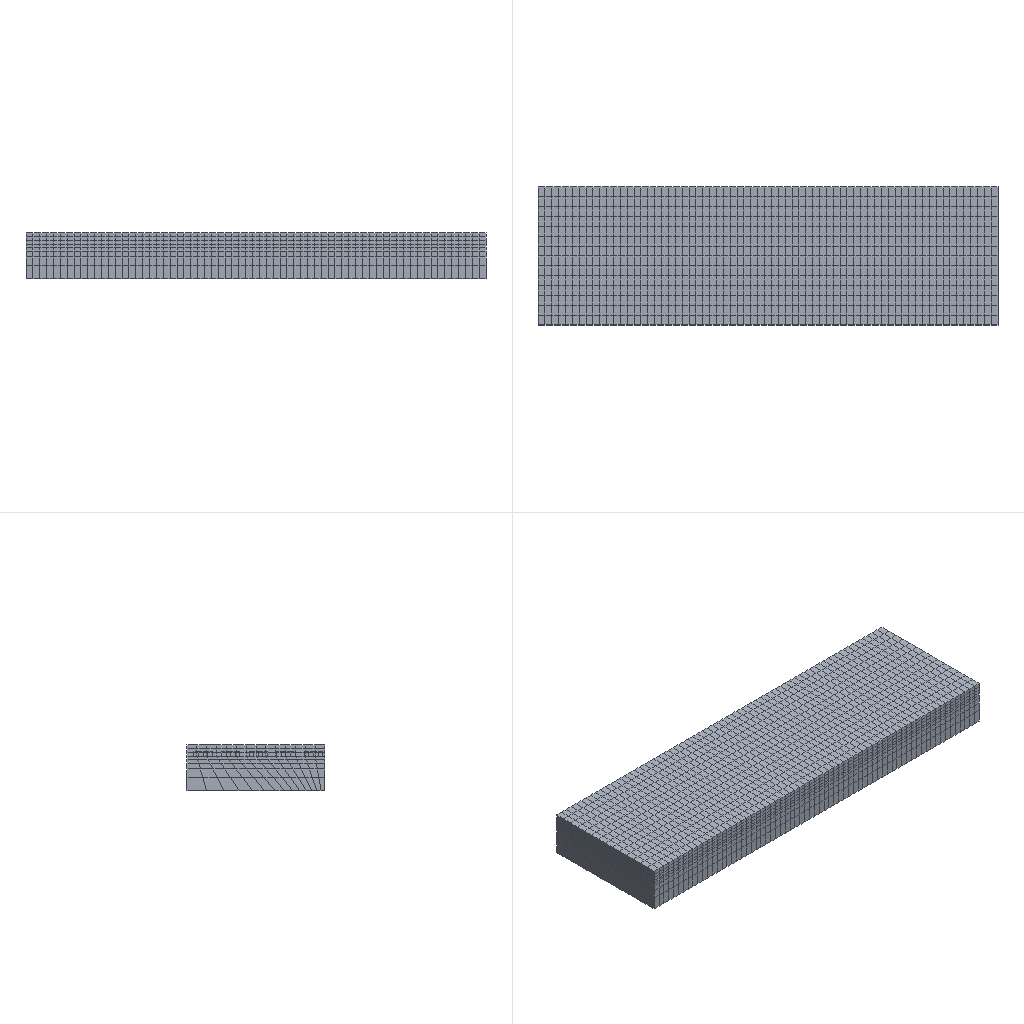Simulation study | abaqus
Set-up summary:
category,name,step,type,value,unit,region
solver,abaqus
solver,version,,,Abaqus/Explicit 2020
units,not stated in the deck,,not stated
analysis,deck,,transient,transient
load_step,Step-1,Step-1,transient
load_step,requested,,,1
mesh,nodes,,,14180
mesh,elements,,,9725
element_type,R3D3,,rigid,228
element_type,R3D4,,rigid,633
element_type,C3D8R,,solid,1360
element_type,EC3D8R,,solid,7504
load,load commands in deck,,count,1
bc,support commands in deck,,count,10
material,BING,,in results
material,COH,,in results
material,WATER,,in results
check,setup vs results,,match,"per instance, exact: element labels, types and connectivity; labels of the nodes the elements use; coordinates of those nodes at SINGLE_PRECISION in 86 of 87 instance(s)"
Abaqus input file, long lists of numbers shortened:
*Heading
** Job name: Job-3 Model name: Model-1-Copy-Copy
** Generated by: Abaqus/CAE 2020
*Preprint, echo=NO, model=NO, history=NO, contact=NO
**
** PARTS
**
*Part, name=aa
*Node
      1,           0.,        -400.,         100.
      2,           0.,        -300.,         100.
** (48 more lines like these left out)
*Element, type=C3D8R
 1, 11, 12, 17, 16,  1,  2,  7,  6
 2, 12, 13, 18, 17,  2,  3,  8,  7
** (14 more lines like these left out)
*Nset, nset=Set-1, generate
  1,  50,   1
*Elset, elset=Set-1, generate
  1,  16,   1
** Section: bing
*Solid Section, elset=Set-1, material=bing
,
*End Part
**
*Part, name=oula
*Node
      1,       10000.,           0.,         750.
      2,       10000.,       -3000.,         750.
** (9178 more lines like these left out)
*Element, type=EC3D8R
   1,  212, 1143, 4033,  615,    1,   13,  511,   46
   2, 1143, 1144, 4034, 4033,   13,   14,  512,  511
** (7502 more lines like these left out)
*Nset, nset=Set-1, generate
    1,  9180,     1
*Elset, elset=Set-1, generate
    1,  7504,     1
** Section: oula
*Eulerian Section, elset=Set-1
water, water-1
*Surface, type=EULERIAN MATERIAL, name=water-1
water-1
*End Part
**
*Part, name=work
*Node
      1,    2.375,   6757.633,   37190.746
      2,    2.375,   6757.633,   40618.258
** (747 more lines like these left out)
*Element, type=R3D4
 1,  1, 21, 64,  4
 2, 21, 22, 63, 64
** (631 more lines like these left out)
*Element, type=R3D3
369,  4, 65,  5
370, 71, 59, 58
** (226 more lines like these left out)
*Node
    750,    2.375,   6959.508,   38910.039
*Nset, nset=work-RefPt_, internal
750,
*Elset, elset=work, generate
   1,  861,    1
*End Part
**
**
** ASSEMBLY
**
*Assembly, name=Assembly
**
*Instance, name=work-1, part=work
37076.822, -1497.625, -5616.383
37076.822, -1497.625, -5616.383, 37077.399, -1498.203, -5616.96,         120.
*End Instance
**
*Instance, name=oula-1, part=oula
          0.,           0.,         250.
*End Instance
**
*Instance, name=aa-1, part=aa
       9600.,       -2550.,        1000.
*End Instance
**
*Instance, name=aa-1-lin-1-2, part=aa
       9600.,       -1950.,        1000.
*End Instance
**
*Instance, name=aa-1-lin-1-3, part=aa
       9600.,       -1350.,        1000.
*End Instance
**
*Instance, name=aa-1-lin-1-4, part=aa
       9600.,        -750.,        1000.
*End Instance
**
*Instance, name=aa-1-lin-1-5, part=aa
       9600.,        -150.,        1000.
*End Instance
**
*Instance, name=aa-1-lin-2-1, part=aa
       9000.,       -2550.,        1000.
*End Instance
**
*Instance, name=aa-1-lin-2-2, part=aa
       9000.,       -1950.,        1000.
*End Instance
**
*Instance, name=aa-1-lin-2-3, part=aa
       9000.,       -1350.,        1000.
*End Instance
**
*Instance, name=aa-1-lin-2-4, part=aa
       9000.,        -750.,        1000.
*End Instance
**
*Instance, name=aa-1-lin-2-5, part=aa
       9000.,        -150.,        1000.
*End Instance
**
*Instance, name=aa-1-lin-3-1, part=aa
       8400.,       -2550.,        1000.
*End Instance
**
*Instance, name=aa-1-lin-3-2, part=aa
       8400.,       -1950.,        1000.
*End Instance
**
*Instance, name=aa-1-lin-3-3, part=aa
       8400.,       -1350.,        1000.
*End Instance
**
*Instance, name=aa-1-lin-3-4, part=aa
       8400.,        -750.,        1000.
*End Instance
**
*Instance, name=aa-1-lin-3-5, part=aa
       8400.,        -150.,        1000.
*End Instance
**
*Instance, name=aa-1-lin-4-1, part=aa
       7800.,       -2550.,        1000.
*End Instance
**
*Instance, name=aa-1-lin-4-2, part=aa
       7800.,       -1950.,        1000.
*End Instance
**
*Instance, name=aa-1-lin-4-3, part=aa
       7800.,       -1350.,        1000.
*End Instance
**
*Instance, name=aa-1-lin-4-4, part=aa
       7800.,        -750.,        1000.
*End Instance
**
*Instance, name=aa-1-lin-4-5, part=aa
       7800.,        -150.,        1000.
*End Instance
**
*Instance, name=aa-1-lin-5-1, part=aa
       7200.,       -2550.,        1000.
*End Instance
**
*Instance, name=aa-1-lin-5-2, part=aa
       7200.,       -1950.,        1000.
*End Instance
**
*Instance, name=aa-1-lin-5-3, part=aa
       7200.,       -1350.,        1000.
*End Instance
**
*Instance, name=aa-1-lin-5-4, part=aa
       7200.,        -750.,        1000.
*End Instance
**
*Instance, name=aa-1-lin-5-5, part=aa
       7200.,        -150.,        1000.
*End Instance
**
*Instance, name=aa-1-lin-6-1, part=aa
       6600.,       -2550.,        1000.
*End Instance
**
*Instance, name=aa-1-lin-6-2, part=aa
       6600.,       -1950.,        1000.
*End Instance
**
*Instance, name=aa-1-lin-6-3, part=aa
       6600.,       -1350.,        1000.
*End Instance
**
*Instance, name=aa-1-lin-6-4, part=aa
       6600.,        -750.,        1000.
*End Instance
**
*Instance, name=aa-1-lin-6-5, part=aa
       6600.,        -150.,        1000.
*End Instance
**
*Instance, name=aa-1-lin-7-1, part=aa
       6000.,       -2550.,        1000.
*End Instance
**
*Instance, name=aa-1-lin-7-2, part=aa
       6000.,       -1950.,        1000.
*End Instance
**
*Instance, name=aa-1-lin-7-3, part=aa
       6000.,       -1350.,        1000.
*End Instance
**
*Instance, name=aa-1-lin-7-4, part=aa
       6000.,        -750.,        1000.
*End Instance
**
*Instance, name=aa-1-lin-7-5, part=aa
       6000.,        -150.,        1000.
*End Instance
**
*Instance, name=aa-1-lin-8-1, part=aa
       5400.,       -2550.,        1000.
*End Instance
**
*Instance, name=aa-1-lin-8-2, part=aa
       5400.,       -1950.,        1000.
*End Instance
**
*Instance, name=aa-1-lin-8-3, part=aa
       5400.,       -1350.,        1000.
*End Instance
**
*Instance, name=aa-1-lin-8-4, part=aa
       5400.,        -750.,        1000.
*End Instance
**
*Instance, name=aa-1-lin-8-5, part=aa
       5400.,        -150.,        1000.
*End Instance
**
*Instance, name=aa-1-lin-9-1, part=aa
       4800.,       -2550.,        1000.
*End Instance
**
*Instance, name=aa-1-lin-9-2, part=aa
       4800.,       -1950.,        1000.
*End Instance
**
*Instance, name=aa-1-lin-9-3, part=aa
       4800.,       -1350.,        1000.
*End Instance
**
*Instance, name=aa-1-lin-9-4, part=aa
       4800.,        -750.,        1000.
*End Instance
**
*Instance, name=aa-1-lin-9-5, part=aa
       4800.,        -150.,        1000.
*End Instance
**
*Instance, name=aa-1-lin-10-1, part=aa
       4200.,       -2550.,        1000.
*End Instance
**
*Instance, name=aa-1-lin-10-2, part=aa
       4200.,       -1950.,        1000.
*End Instance
**
*Instance, name=aa-1-lin-10-3, part=aa
       4200.,       -1350.,        1000.
*End Instance
**
*Instance, name=aa-1-lin-10-4, part=aa
       4200.,        -750.,        1000.
*End Instance
**
*Instance, name=aa-1-lin-10-5, part=aa
       4200.,        -150.,        1000.
*End Instance
**
*Instance, name=aa-1-lin-11-1, part=aa
       3600.,       -2550.,        1000.
*End Instance
**
*Instance, name=aa-1-lin-11-2, part=aa
       3600.,       -1950.,        1000.
*End Instance
**
*Instance, name=aa-1-lin-11-3, part=aa
       3600.,       -1350.,        1000.
*End Instance
**
*Instance, name=aa-1-lin-11-4, part=aa
       3600.,        -750.,        1000.
*End Instance
**
*Instance, name=aa-1-lin-11-5, part=aa
       3600.,        -150.,        1000.
*End Instance
**
*Instance, name=aa-1-lin-12-1, part=aa
       3000.,       -2550.,        1000.
*End Instance
**
*Instance, name=aa-1-lin-12-2, part=aa
       3000.,       -1950.,        1000.
*End Instance
**
*Instance, name=aa-1-lin-12-3, part=aa
       3000.,       -1350.,        1000.
*End Instance
**
*Instance, name=aa-1-lin-12-4, part=aa
       3000.,        -750.,        1000.
*End Instance
**
*Instance, name=aa-1-lin-12-5, part=aa
       3000.,        -150.,        1000.
*End Instance
**
*Instance, name=aa-1-lin-13-1, part=aa
       2400.,       -2550.,        1000.
*End Instance
**
*Instance, name=aa-1-lin-13-2, part=aa
       2400.,       -1950.,        1000.
*End Instance
**
*Instance, name=aa-1-lin-13-3, part=aa
       2400.,       -1350.,        1000.
*End Instance
**
*Instance, name=aa-1-lin-13-4, part=aa
       2400.,        -750.,        1000.
*End Instance
**
*Instance, name=aa-1-lin-13-5, part=aa
       2400.,        -150.,        1000.
*End Instance
**
*Instance, name=aa-1-lin-14-1, part=aa
       1800.,       -2550.,        1000.
*End Instance
**
*Instance, name=aa-1-lin-14-2, part=aa
       1800.,       -1950.,        1000.
*End Instance
**
*Instance, name=aa-1-lin-14-3, part=aa
       1800.,       -1350.,        1000.
*End Instance
**
*Instance, name=aa-1-lin-14-4, part=aa
       1800.,        -750.,        1000.
*End Instance
**
*Instance, name=aa-1-lin-14-5, part=aa
       1800.,        -150.,        1000.
*End Instance
**
*Instance, name=aa-1-lin-15-1, part=aa
       1200.,       -2550.,        1000.
*End Instance
**
*Instance, name=aa-1-lin-15-2, part=aa
       1200.,       -1950.,        1000.
*End Instance
**
*Instance, name=aa-1-lin-15-3, part=aa
       1200.,       -1350.,        1000.
*End Instance
**
*Instance, name=aa-1-lin-15-4, part=aa
       1200.,        -750.,        1000.
*End Instance
**
*Instance, name=aa-1-lin-15-5, part=aa
       1200.,        -150.,        1000.
*End Instance
**
*Instance, name=aa-1-lin-16-1, part=aa
        600.,       -2550.,        1000.
*End Instance
**
*Instance, name=aa-1-lin-16-2, part=aa
        600.,       -1950.,        1000.
*End Instance
**
*Instance, name=aa-1-lin-16-3, part=aa
        600.,       -1350.,        1000.
*End Instance
**
*Instance, name=aa-1-lin-16-4, part=aa
        600.,        -750.,        1000.
*End Instance
**
*Instance, name=aa-1-lin-16-5, part=aa
        600.,        -150.,        1000.
*End Instance
**
*Instance, name=aa-1-lin-17-1, part=aa
          0.,       -2550.,        1000.
*End Instance
**
*Instance, name=aa-1-lin-17-2, part=aa
          0.,       -1950.,        1000.
*End Instance
**
*Instance, name=aa-1-lin-17-3, part=aa
          0.,       -1350.,        1000.
*End Instance
**
*Instance, name=aa-1-lin-17-4, part=aa
          0.,        -750.,        1000.
*End Instance
**
*Instance, name=aa-1-lin-17-5, part=aa
          0.,        -150.,        1000.
*End Instance
**
*Nset, nset=Set-1, instance=oula-1
    1,    2,    3,    4,    5,    6,    7,    8,   13,   14,   15,   16,   17,   18,   19,   20
   21,   22,   23,   24,   25,   26,   27,   28,   29,   30,   31,   32,   33,   34,   35,   36
** (381 more lines like these left out)
*Elset, elset=Set-1, instance=oula-1, generate
    1,  4690,     1
*Nset, nset=Set-3, instance=oula-1
    1,    2,    3,    4,    5,    6,    7,    8,    9,   10,   11,   12,   26,   27,   28,   29
   43,   44,   45,   46,   60,   61,   62,   63,   77,   78,   79,   80,   81,   82,   83,   84
** (75 more lines like these left out)
*Elset, elset=Set-3, instance=oula-1
    1,   14,   15,   28,   29,   42,   43,   56,   57,   70,   71,   84,   85,   98,   99,  112
  113,  126,  127,  140,  141,  154,  155,  168,  169,  182,  183,  196,  197,  210,  211,  224
** (65 more lines like these left out)
*Nset, nset=Set-4, instance=oula-1
    3,    4,    6,    7,   30,   31,   32,   33,   34,   35,   36,   37,   38,   39,   40,   41
   42,   64,   65,   66,   67,   68,   69,   70,   71,   72,   73,   74,   75,   76,   81,   82
** (62 more lines like these left out)
*Elset, elset=Set-4, instance=oula-1
   57,   58,   59,   60,   61,   62,   63,   64,   65,   66,   67,   68,   69,   70,  127,  128
  129,  130,  131,  132,  133,  134,  135,  136,  137,  138,  139,  140,  197,  198,  199,  200
** (57 more lines like these left out)
*Nset, nset=Set-5, instance=oula-1
   1,   2,   3,   4,  13,  14,  15,  16,  17,  18,  19,  20,  21,  22,  23,  24
  25,  26,  27,  28,  29,  30,  31,  32,  33,  34,  35,  36,  37,  38,  39,  40
** (4 more lines like these left out)
*Elset, elset=Set-5, instance=oula-1, generate
  1,  70,   1
*Nset, nset=Set-6, instance=work-1
 750,
*Nset, nset=Set-7, instance=aa-1
  1,  6, 11, 16, 21, 26, 31, 36, 41, 42, 43, 44, 45, 46, 47, 48
 49, 50
*Nset, nset=Set-7, instance=aa-1-lin-1-2, generate
 41,  50,   1
*Nset, nset=Set-7, instance=aa-1-lin-1-3, generate
 41,  50,   1
*Nset, nset=Set-7, instance=aa-1-lin-1-5
  5, 10, 15, 20, 25, 30, 35, 40, 41, 42, 43, 44, 45, 46, 47, 48
 49, 50
*Nset, nset=Set-7, instance=aa-1-lin-5-5, generate
  5,  50,   5
*Nset, nset=Set-7, instance=aa-1-lin-9-1, generate
  1,  46,   5
*Nset, nset=Set-7, instance=aa-1-lin-13-5, generate
  5,  50,   5
*Nset, nset=Set-7, instance=aa-1-lin-17-1, generate
  1,  46,   5
*Nset, nset=Set-7, instance=aa-1-lin-5-1, generate
  1,  46,   5
*Nset, nset=Set-7, instance=aa-1-lin-9-5, generate
  5,  50,   5
*Nset, nset=Set-7, instance=aa-1-lin-13-1, generate
  1,  46,   5
*Nset, nset=Set-7, instance=aa-1-lin-17-5, generate
  5,  50,   5
*Nset, nset=Set-7, instance=aa-1-lin-3-1, generate
  1,  46,   5
*Nset, nset=Set-7, instance=aa-1-lin-7-5, generate
  5,  50,   5
*Nset, nset=Set-7, instance=aa-1-lin-15-5, generate
  5,  50,   5
*Nset, nset=Set-7, instance=aa-1-lin-11-1, generate
  1,  46,   5
*Nset, nset=Set-7, instance=aa-1-lin-3-5, generate
  5,  50,   5
*Nset, nset=Set-7, instance=aa-1-lin-7-1, generate
  1,  46,   5
*Nset, nset=Set-7, instance=aa-1-lin-11-5, generate
  5,  50,   5
*Nset, nset=Set-7, instance=aa-1-lin-15-1, generate
  1,  46,   5
*Nset, nset=Set-7, instance=aa-1-lin-1-4, generate
 41,  50,   1
*Nset, nset=Set-7, instance=aa-1-lin-2-1, generate
  1,  46,   5
*Nset, nset=Set-7, instance=aa-1-lin-2-5, generate
  5,  50,   5
*Nset, nset=Set-7, instance=aa-1-lin-6-1, generate
  1,  46,   5
*Nset, nset=Set-7, instance=aa-1-lin-10-5, generate
  5,  50,   5
*Nset, nset=Set-7, instance=aa-1-lin-14-1, generate
  1,  46,   5
*Nset, nset=Set-7, instance=aa-1-lin-6-5, generate
  5,  50,   5
*Nset, nset=Set-7, instance=aa-1-lin-10-1, generate
  1,  46,   5
*Nset, nset=Set-7, instance=aa-1-lin-14-5, generate
  5,  50,   5
*Nset, nset=Set-7, instance=aa-1-lin-4-1, generate
  1,  46,   5
*Nset, nset=Set-7, instance=aa-1-lin-4-5, generate
  5,  50,   5
*Nset, nset=Set-7, instance=aa-1-lin-12-5, generate
  5,  50,   5
*Nset, nset=Set-7, instance=aa-1-lin-16-1, generate
  1,  46,   5
*Nset, nset=Set-7, instance=aa-1-lin-8-1, generate
  1,  46,   5
*Nset, nset=Set-7, instance=aa-1-lin-8-5, generate
  5,  50,   5
*Nset, nset=Set-7, instance=aa-1-lin-16-5, generate
  5,  50,   5
*Nset, nset=Set-7, instance=aa-1-lin-12-1, generate
  1,  46,   5
*Elset, elset=Set-7, instance=aa-1
  1,  5,  9, 13, 14, 15, 16
*Elset, elset=Set-7, instance=aa-1-lin-1-2, generate
 13,  16,   1
*Elset, elset=Set-7, instance=aa-1-lin-1-3, generate
 13,  16,   1
*Elset, elset=Set-7, instance=aa-1-lin-1-5
  4,  8, 12, 13, 14, 15, 16
*Elset, elset=Set-7, instance=aa-1-lin-5-5, generate
  4,  16,   4
*Elset, elset=Set-7, instance=aa-1-lin-9-1, generate
  1,  13,   4
*Elset, elset=Set-7, instance=aa-1-lin-13-5, generate
  4,  16,   4
*Elset, elset=Set-7, instance=aa-1-lin-17-1, generate
  1,  13,   4
*Elset, elset=Set-7, instance=aa-1-lin-5-1, generate
  1,  13,   4
*Elset, elset=Set-7, instance=aa-1-lin-9-5, generate
  4,  16,   4
*Elset, elset=Set-7, instance=aa-1-lin-13-1, generate
  1,  13,   4
*Elset, elset=Set-7, instance=aa-1-lin-17-5, generate
  4,  16,   4
*Elset, elset=Set-7, instance=aa-1-lin-3-1, generate
  1,  13,   4
*Elset, elset=Set-7, instance=aa-1-lin-7-5, generate
  4,  16,   4
*Elset, elset=Set-7, instance=aa-1-lin-15-5, generate
  4,  16,   4
*Elset, elset=Set-7, instance=aa-1-lin-11-1, generate
  1,  13,   4
*Elset, elset=Set-7, instance=aa-1-lin-3-5, generate
  4,  16,   4
*Elset, elset=Set-7, instance=aa-1-lin-7-1, generate
  1,  13,   4
*Elset, elset=Set-7, instance=aa-1-lin-11-5, generate
  4,  16,   4
*Elset, elset=Set-7, instance=aa-1-lin-15-1, generate
  1,  13,   4
*Elset, elset=Set-7, instance=aa-1-lin-1-4, generate
 13,  16,   1
*Elset, elset=Set-7, instance=aa-1-lin-2-1, generate
  1,  13,   4
*Elset, elset=Set-7, instance=aa-1-lin-2-5, generate
  4,  16,   4
*Elset, elset=Set-7, instance=aa-1-lin-6-1, generate
  1,  13,   4
*Elset, elset=Set-7, instance=aa-1-lin-10-5, generate
  4,  16,   4
*Elset, elset=Set-7, instance=aa-1-lin-14-1, generate
  1,  13,   4
*Elset, elset=Set-7, instance=aa-1-lin-6-5, generate
  4,  16,   4
*Elset, elset=Set-7, instance=aa-1-lin-10-1, generate
  1,  13,   4
*Elset, elset=Set-7, instance=aa-1-lin-14-5, generate
  4,  16,   4
*Elset, elset=Set-7, instance=aa-1-lin-4-1, generate
  1,  13,   4
*Elset, elset=Set-7, instance=aa-1-lin-4-5, generate
  4,  16,   4
*Elset, elset=Set-7, instance=aa-1-lin-12-5, generate
  4,  16,   4
*Elset, elset=Set-7, instance=aa-1-lin-16-1, generate
  1,  13,   4
*Elset, elset=Set-7, instance=aa-1-lin-8-1, generate
  1,  13,   4
*Elset, elset=Set-7, instance=aa-1-lin-8-5, generate
  4,  16,   4
*Elset, elset=Set-7, instance=aa-1-lin-16-5, generate
  4,  16,   4
*Elset, elset=Set-7, instance=aa-1-lin-12-1, generate
  1,  13,   4
*Rigid Body, ref node=work-1.work-RefPt_, elset=work-1.work
*End Assembly
**
** MATERIALS
**
*Material, name=bing
*Brittle Cracking
100.,   0.
250., 0.05
*Brittle Shear
1.,  0.
0., 0.1
*Brittle Failure
 0.01,
*Density
 9.2e-10,
*Elastic
1000., 0.3
*Material, name=coh
*Damage Initiation, criterion=MAXS
10.,10.,10.
*Damage Evolution, type=DISPLACEMENT
 1e-11,
*Density
 9.2e-10,
*Elastic, type=TRACTION
1000.,1000.,1000.
*Material, name=water
*Density
 1e-09,
*Eos, type=USUP
1483.,0.,0.
*Viscosity
 0.01,
**
** INTERACTION PROPERTIES
**
*Surface Interaction, name=IntProp-1
*Friction
 0.2,
*Surface Behavior, pressure-overclosure=HARD
**
** PREDEFINED FIELDS
**
** Name: Predefined Field-1   Type: Material assignment
*Initial Conditions, type=VOLUME FRACTION
Set-1, oula-1.water-1, 1.
** ----------------------------------------------------------------
**
** STEP: Step-1
**
*Step, name=Step-1, nlgeom=YES
*Dynamic, Explicit
, 1.
*Bulk Viscosity
0.06, 1.2
** Mass Scaling: Semi-Automatic
**               Whole Model
*Fixed Mass Scaling, factor=5000.
**
** BOUNDARY CONDITIONS
**
** Name: BC-1 Type: 对称/反对称/完全固定
*Boundary
Set-7, ENCASTRE
** Name: [REDACTED] : Speed/Angular velocity
*Boundary, type=VELOCITY
Set-4, 3, 3
** Name: [REDACTED] : Speed/Angular velocity
*Boundary, type=VELOCITY
Set-5, 1, 1
** Name: [REDACTED] : Speed/Angular velocity
*Boundary, type=VELOCITY
Set-3, 2, 2
** Name: [REDACTED] : Speed/Angular velocity
*Boundary, type=VELOCITY
Set-6, 1, 1, 8300.
Set-6, 2, 2
Set-6, 3, 3
Set-6, 4, 4
Set-6, 5, 5
Set-6, 6, 6
**
** INTERACTIONS
**
** Interaction: Int-1
*Contact, op=NEW
*Contact Inclusions, ALL EXTERIOR
*Contact Property Assignment
 ,  , IntProp-1
**
** OUTPUT REQUESTS
**
*Restart, write, number interval=1, time marks=NO
**
** FIELD OUTPUT: F-Output-1
**
*Output, field, number interval=50
*Node Output
A, CF, RF, RM, RT, U, V
*Element Output, directions=YES
DENSITYVAVG, E, EVF, EVOL, LE, MISES, MISESMAX, PE, PEEQ, PEEQVAVG, PEVAVG, S, SF, SSAVG, STATUS, SVAVG
SVOL, TSHR
*Contact Output
CDISP, CSTRESS
**
** HISTORY OUTPUT: H-Output-1
**
*Output, history, time interval=5e-05
*Node Output, nset=Set-6
RF1, RF2, RF3
*End Step
Results summary:
result,step,Step-1,completed,increments=16881 time=1.0/1.0
result,analysis,,,transient
result,last_loadstep,,,1
result,primary field,,,U
result,reaction total,,FX,444177.746,model units
result,reaction total,,FY,1794968.174,model units
result,reaction total,,FZ,178896.077,model units